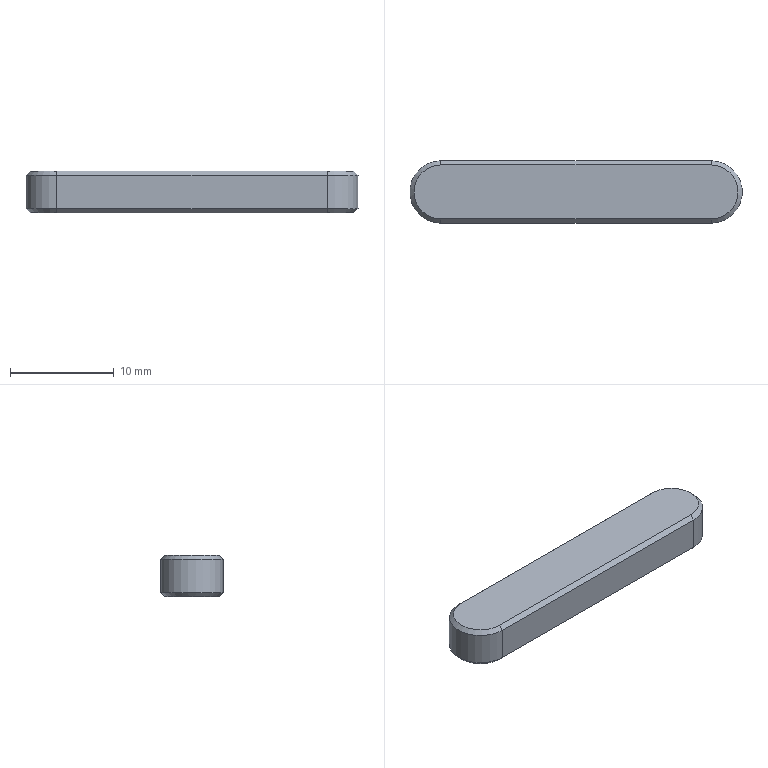Part | STEP file | ISO 2491 - A  6 x 4 x 32 | 1 solid | 14 faces | box 32 x 6 x 4 mm | volume 725.895 mm3 | plane 8 | cone 4 | cylinder 2 | commonest cylinder face diameters 6 x2
STEP:
#1=CARTESIAN_POINT('',(0.,0.,0.));
#2=DIRECTION('',(0.,0.,1.));
#3=DIRECTION('',(1.,0.,0.));
#4=AXIS2_PLACEMENT_3D('',#1,#2,#3);
#5=CARTESIAN_POINT('',(29.,-2.6,-2.5));
#6=VERTEX_POINT('',#5);
#7=CARTESIAN_POINT('',(29.,-3.,-2.1));
#8=VERTEX_POINT('',#7);
#9=CARTESIAN_POINT('',(29.,-2.6,-2.5));
#10=DIRECTION('',(0.,-0.7071,0.7071));
#11=VECTOR('',#10,1.);
#12=LINE('',#9,#11);
#13=CARTESIAN_POINT('',(9.5,-2.8,-2.3));
#14=DIRECTION('',(0.,-0.7071,-0.7071));
#15=DIRECTION('',(-1.,0.,0.));
#16=AXIS2_PLACEMENT_3D('',#13,#14,#15);
#17=PLANE('',#16);
#18=CARTESIAN_POINT('',(-19.5,0.2828));
#19=DIRECTION('',(0.,-1.));
#20=VECTOR('',#19,1.);
#21=LINE('',#18,#20);
#22=(GEOMETRIC_REPRESENTATION_CONTEXT(2)PARAMETRIC_REPRESENTATION_CONTEXT()REPRESENTATION_CONTEXT('',''));
#23=DEFINITIONAL_REPRESENTATION('',(#21),#22);
#24=PCURVE('',#17,#23);
#25=CARTESIAN_POINT('',(29.,0.,-2.3));
#26=DIRECTION('',(0.,0.,1.));
#27=DIRECTION('',(0.,1.,0.));
#28=AXIS2_PLACEMENT_3D('',#25,#26,#27);
#29=CONICAL_SURFACE('',#28,2.8,0.7854);
#30=CARTESIAN_POINT('',(3.142,-0.2));
#31=DIRECTION('',(0.,1.));
#32=VECTOR('',#31,1.);
#33=LINE('',#30,#32);
#34=(GEOMETRIC_REPRESENTATION_CONTEXT(2)PARAMETRIC_REPRESENTATION_CONTEXT()REPRESENTATION_CONTEXT('',''));
#35=DEFINITIONAL_REPRESENTATION('',(#33),#34);
#36=PCURVE('',#29,#35);
#37=SURFACE_CURVE('',#12,(#24,#36),.PCURVE_S1.);
#38=EDGE_CURVE('',#6,#8,#37,.T.);
#39=ORIENTED_EDGE('',*,*,#38,.T.);
#40=CARTESIAN_POINT('',(3.,-3.,-2.1));
#41=VERTEX_POINT('',#40);
#42=CARTESIAN_POINT('',(9.5,-3.,-2.1));
#43=DIRECTION('',(-1.,0.,0.));
#44=VECTOR('',#43,1.);
#45=LINE('',#42,#44);
#46=CARTESIAN_POINT('',(0.,-0.2828));
#47=DIRECTION('',(1.,0.));
#48=VECTOR('',#47,1.);
#49=LINE('',#46,#48);
#50=(GEOMETRIC_REPRESENTATION_CONTEXT(2)PARAMETRIC_REPRESENTATION_CONTEXT()REPRESENTATION_CONTEXT('',''));
#51=DEFINITIONAL_REPRESENTATION('',(#49),#50);
#52=PCURVE('',#17,#51);
#53=CARTESIAN_POINT('',(3.,-3.,0.));
#54=DIRECTION('',(0.,-1.,0.));
#55=DIRECTION('',(0.,0.,-1.));
#56=AXIS2_PLACEMENT_3D('',#53,#54,#55);
#57=PLANE('',#56);
#58=CARTESIAN_POINT('',(2.1,6.5));
#59=DIRECTION('',(0.,-1.));
#60=VECTOR('',#59,1.);
#61=LINE('',#58,#60);
#62=(GEOMETRIC_REPRESENTATION_CONTEXT(2)PARAMETRIC_REPRESENTATION_CONTEXT()REPRESENTATION_CONTEXT('',''));
#63=DEFINITIONAL_REPRESENTATION('',(#61),#62);
#64=PCURVE('',#57,#63);
#65=SURFACE_CURVE('',#45,(#52,#64),.PCURVE_S1.);
#66=EDGE_CURVE('',#8,#41,#65,.T.);
#67=ORIENTED_EDGE('',*,*,#66,.T.);
#68=CARTESIAN_POINT('',(3.,-2.6,-2.5));
#69=VERTEX_POINT('',#68);
#70=CARTESIAN_POINT('',(3.,-3.,-2.1));
#71=DIRECTION('',(0.,0.7071,-0.7071));
#72=VECTOR('',#71,1.);
#73=LINE('',#70,#72);
#74=CARTESIAN_POINT('',(6.5,-0.2828));
#75=DIRECTION('',(0.,1.));
#76=VECTOR('',#75,1.);
#77=LINE('',#74,#76);
#78=(GEOMETRIC_REPRESENTATION_CONTEXT(2)PARAMETRIC_REPRESENTATION_CONTEXT()REPRESENTATION_CONTEXT('',''));
#79=DEFINITIONAL_REPRESENTATION('',(#77),#78);
#80=PCURVE('',#17,#79);
#81=CARTESIAN_POINT('',(3.,0.,-2.3));
#82=DIRECTION('',(0.,0.,1.));
#83=DIRECTION('',(0.,-1.,0.));
#84=AXIS2_PLACEMENT_3D('',#81,#82,#83);
#85=CONICAL_SURFACE('',#84,2.8,0.7854);
#86=CARTESIAN_POINT('',(6.283,0.2));
#87=DIRECTION('',(0.,-1.));
#88=VECTOR('',#87,1.);
#89=LINE('',#86,#88);
#90=(GEOMETRIC_REPRESENTATION_CONTEXT(2)PARAMETRIC_REPRESENTATION_CONTEXT()REPRESENTATION_CONTEXT('',''));
#91=DEFINITIONAL_REPRESENTATION('',(#89),#90);
#92=PCURVE('',#85,#91);
#93=SURFACE_CURVE('',#73,(#80,#92),.PCURVE_S1.);
#94=EDGE_CURVE('',#41,#69,#93,.T.);
#95=ORIENTED_EDGE('',*,*,#94,.T.);
#96=CARTESIAN_POINT('',(9.5,-2.6,-2.5));
#97=DIRECTION('',(1.,0.,0.));
#98=VECTOR('',#97,1.);
#99=LINE('',#96,#98);
#100=CARTESIAN_POINT('',(0.,0.2828));
#101=DIRECTION('',(-1.,0.));
#102=VECTOR('',#101,1.);
#103=LINE('',#100,#102);
#104=(GEOMETRIC_REPRESENTATION_CONTEXT(2)PARAMETRIC_REPRESENTATION_CONTEXT()REPRESENTATION_CONTEXT('',''));
#105=DEFINITIONAL_REPRESENTATION('',(#103),#104);
#106=PCURVE('',#17,#105);
#107=CARTESIAN_POINT('',(16.,0.,-2.5));
#108=DIRECTION('',(0.,0.,1.));
#109=DIRECTION('',(1.,0.,0.));
#110=AXIS2_PLACEMENT_3D('',#107,#108,#109);
#111=PLANE('',#110);
#112=CARTESIAN_POINT('',(-6.5,-2.6));
#113=DIRECTION('',(1.,0.));
#114=VECTOR('',#113,1.);
#115=LINE('',#112,#114);
#116=(GEOMETRIC_REPRESENTATION_CONTEXT(2)PARAMETRIC_REPRESENTATION_CONTEXT()REPRESENTATION_CONTEXT('',''));
#117=DEFINITIONAL_REPRESENTATION('',(#115),#116);
#118=PCURVE('',#111,#117);
#119=SURFACE_CURVE('',#99,(#106,#118),.PCURVE_S1.);
#120=EDGE_CURVE('',#69,#6,#119,.T.);
#121=ORIENTED_EDGE('',*,*,#120,.T.);
#122=EDGE_LOOP('',(#39,#67,#95,#121));
#123=FACE_BOUND('',#122,.T.);
#124=ADVANCED_FACE('',(#123),#17,.T.);
#125=CARTESIAN_POINT('',(29.,2.6,-2.5));
#126=VERTEX_POINT('',#125);
#127=CARTESIAN_POINT('',(29.,3.,-2.1));
#128=VERTEX_POINT('',#127);
#129=CARTESIAN_POINT('',(29.,2.6,-2.5));
#130=DIRECTION('',(0.,0.7071,0.7071));
#131=VECTOR('',#130,1.);
#132=LINE('',#129,#131);
#133=CARTESIAN_POINT('',(6.283,-0.2));
#134=DIRECTION('',(0.,1.));
#135=VECTOR('',#134,1.);
#136=LINE('',#133,#135);
#137=(GEOMETRIC_REPRESENTATION_CONTEXT(2)PARAMETRIC_REPRESENTATION_CONTEXT()REPRESENTATION_CONTEXT('',''));
#138=DEFINITIONAL_REPRESENTATION('',(#136),#137);
#139=PCURVE('',#29,#138);
#140=CARTESIAN_POINT('',(22.5,2.8,-2.3));
#141=DIRECTION('',(0.,0.7071,-0.7071));
#142=DIRECTION('',(-1.,0.,0.));
#143=AXIS2_PLACEMENT_3D('',#140,#141,#142);
#144=PLANE('',#143);
#145=CARTESIAN_POINT('',(-6.5,-0.2828));
#146=DIRECTION('',(0.,1.));
#147=VECTOR('',#146,1.);
#148=LINE('',#145,#147);
#149=(GEOMETRIC_REPRESENTATION_CONTEXT(2)PARAMETRIC_REPRESENTATION_CONTEXT()REPRESENTATION_CONTEXT('',''));
#150=DEFINITIONAL_REPRESENTATION('',(#148),#149);
#151=PCURVE('',#144,#150);
#152=SURFACE_CURVE('',#132,(#139,#151),.PCURVE_S1.);
#153=EDGE_CURVE('',#126,#128,#152,.T.);
#154=ORIENTED_EDGE('',*,*,#153,.T.);
#155=CARTESIAN_POINT('',(29.,0.,-2.1));
#156=DIRECTION('',(0.,0.,-1.));
#157=DIRECTION('',(0.,1.,0.));
#158=AXIS2_PLACEMENT_3D('',#155,#156,#157);
#159=CIRCLE('',#158,3.);
#160=CARTESIAN_POINT('',(6.283,0.2));
#161=DIRECTION('',(-1.,0.));
#162=VECTOR('',#161,1.);
#163=LINE('',#160,#162);
#164=(GEOMETRIC_REPRESENTATION_CONTEXT(2)PARAMETRIC_REPRESENTATION_CONTEXT()REPRESENTATION_CONTEXT('',''));
#165=DEFINITIONAL_REPRESENTATION('',(#163),#164);
#166=PCURVE('',#29,#165);
#167=CARTESIAN_POINT('',(29.,0.,0.));
#168=DIRECTION('',(0.,0.,-1.));
#169=DIRECTION('',(0.,1.,0.));
#170=AXIS2_PLACEMENT_3D('',#167,#168,#169);
#171=CYLINDRICAL_SURFACE('',#170,3.);
#172=CARTESIAN_POINT('',(0.,2.1));
#173=DIRECTION('',(1.,0.));
#174=VECTOR('',#173,1.);
#175=LINE('',#172,#174);
#176=(GEOMETRIC_REPRESENTATION_CONTEXT(2)PARAMETRIC_REPRESENTATION_CONTEXT()REPRESENTATION_CONTEXT('',''));
#177=DEFINITIONAL_REPRESENTATION('',(#175),#176);
#178=PCURVE('',#171,#177);
#179=SURFACE_CURVE('',#159,(#166,#178),.PCURVE_S1.);
#180=EDGE_CURVE('',#128,#8,#179,.T.);
#181=ORIENTED_EDGE('',*,*,#180,.T.);
#182=ORIENTED_EDGE('',*,*,#38,.F.);
#183=CARTESIAN_POINT('',(29.,0.,-2.5));
#184=DIRECTION('',(0.,0.,1.));
#185=DIRECTION('',(0.,1.,0.));
#186=AXIS2_PLACEMENT_3D('',#183,#184,#185);
#187=CIRCLE('',#186,2.6);
#188=CARTESIAN_POINT('',(0.,-0.2));
#189=DIRECTION('',(1.,0.));
#190=VECTOR('',#189,1.);
#191=LINE('',#188,#190);
#192=(GEOMETRIC_REPRESENTATION_CONTEXT(2)PARAMETRIC_REPRESENTATION_CONTEXT()REPRESENTATION_CONTEXT('',''));
#193=DEFINITIONAL_REPRESENTATION('',(#191),#192);
#194=PCURVE('',#29,#193);
#195=CARTESIAN_POINT('',(13.,0.));
#196=DIRECTION('',(0.,1.));
#197=AXIS2_PLACEMENT_2D('',#195,#196);
#198=CIRCLE('',#197,2.6);
#199=(GEOMETRIC_REPRESENTATION_CONTEXT(2)PARAMETRIC_REPRESENTATION_CONTEXT()REPRESENTATION_CONTEXT('',''));
#200=DEFINITIONAL_REPRESENTATION('',(#198),#199);
#201=PCURVE('',#111,#200);
#202=SURFACE_CURVE('',#187,(#194,#201),.PCURVE_S1.);
#203=EDGE_CURVE('',#6,#126,#202,.T.);
#204=ORIENTED_EDGE('',*,*,#203,.T.);
#205=EDGE_LOOP('',(#154,#181,#182,#204));
#206=FACE_BOUND('',#205,.T.);
#207=ADVANCED_FACE('',(#206),#29,.T.);
#208=CARTESIAN_POINT('',(3.,3.,-2.1));
#209=VERTEX_POINT('',#208);
#210=CARTESIAN_POINT('',(3.,2.6,-2.5));
#211=VERTEX_POINT('',#210);
#212=CARTESIAN_POINT('',(3.,3.,-2.1));
#213=DIRECTION('',(0.,-0.7071,-0.7071));
#214=VECTOR('',#213,1.);
#215=LINE('',#212,#214);
#216=CARTESIAN_POINT('',(3.142,0.2));
#217=DIRECTION('',(0.,-1.));
#218=VECTOR('',#217,1.);
#219=LINE('',#216,#218);
#220=(GEOMETRIC_REPRESENTATION_CONTEXT(2)PARAMETRIC_REPRESENTATION_CONTEXT()REPRESENTATION_CONTEXT('',''));
#221=DEFINITIONAL_REPRESENTATION('',(#219),#220);
#222=PCURVE('',#85,#221);
#223=CARTESIAN_POINT('',(19.5,0.2828));
#224=DIRECTION('',(0.,-1.));
#225=VECTOR('',#224,1.);
#226=LINE('',#223,#225);
#227=(GEOMETRIC_REPRESENTATION_CONTEXT(2)PARAMETRIC_REPRESENTATION_CONTEXT()REPRESENTATION_CONTEXT('',''));
#228=DEFINITIONAL_REPRESENTATION('',(#226),#227);
#229=PCURVE('',#144,#228);
#230=SURFACE_CURVE('',#215,(#222,#229),.PCURVE_S1.);
#231=EDGE_CURVE('',#209,#211,#230,.T.);
#232=ORIENTED_EDGE('',*,*,#231,.T.);
#233=CARTESIAN_POINT('',(3.,0.,-2.5));
#234=DIRECTION('',(0.,0.,1.));
#235=DIRECTION('',(0.,-1.,0.));
#236=AXIS2_PLACEMENT_3D('',#233,#234,#235);
#237=CIRCLE('',#236,2.6);
#238=CARTESIAN_POINT('',(0.,-0.2));
#239=DIRECTION('',(1.,0.));
#240=VECTOR('',#239,1.);
#241=LINE('',#238,#240);
#242=(GEOMETRIC_REPRESENTATION_CONTEXT(2)PARAMETRIC_REPRESENTATION_CONTEXT()REPRESENTATION_CONTEXT('',''));
#243=DEFINITIONAL_REPRESENTATION('',(#241),#242);
#244=PCURVE('',#85,#243);
#245=CARTESIAN_POINT('',(-13.,0.));
#246=DIRECTION('',(0.,-1.));
#247=AXIS2_PLACEMENT_2D('',#245,#246);
#248=CIRCLE('',#247,2.6);
#249=(GEOMETRIC_REPRESENTATION_CONTEXT(2)PARAMETRIC_REPRESENTATION_CONTEXT()REPRESENTATION_CONTEXT('',''));
#250=DEFINITIONAL_REPRESENTATION('',(#248),#249);
#251=PCURVE('',#111,#250);
#252=SURFACE_CURVE('',#237,(#244,#251),.PCURVE_S1.);
#253=EDGE_CURVE('',#211,#69,#252,.T.);
#254=ORIENTED_EDGE('',*,*,#253,.T.);
#255=ORIENTED_EDGE('',*,*,#94,.F.);
#256=CARTESIAN_POINT('',(3.,0.,-2.1));
#257=DIRECTION('',(0.,0.,-1.));
#258=DIRECTION('',(0.,-1.,0.));
#259=AXIS2_PLACEMENT_3D('',#256,#257,#258);
#260=CIRCLE('',#259,3.);
#261=CARTESIAN_POINT('',(6.283,0.2));
#262=DIRECTION('',(-1.,0.));
#263=VECTOR('',#262,1.);
#264=LINE('',#261,#263);
#265=(GEOMETRIC_REPRESENTATION_CONTEXT(2)PARAMETRIC_REPRESENTATION_CONTEXT()REPRESENTATION_CONTEXT('',''));
#266=DEFINITIONAL_REPRESENTATION('',(#264),#265);
#267=PCURVE('',#85,#266);
#268=CARTESIAN_POINT('',(3.,0.,0.));
#269=DIRECTION('',(0.,0.,-1.));
#270=DIRECTION('',(0.,-1.,0.));
#271=AXIS2_PLACEMENT_3D('',#268,#269,#270);
#272=CYLINDRICAL_SURFACE('',#271,3.);
#273=CARTESIAN_POINT('',(0.,2.1));
#274=DIRECTION('',(1.,0.));
#275=VECTOR('',#274,1.);
#276=LINE('',#273,#275);
#277=(GEOMETRIC_REPRESENTATION_CONTEXT(2)PARAMETRIC_REPRESENTATION_CONTEXT()REPRESENTATION_CONTEXT('',''));
#278=DEFINITIONAL_REPRESENTATION('',(#276),#277);
#279=PCURVE('',#272,#278);
#280=SURFACE_CURVE('',#260,(#267,#279),.PCURVE_S1.);
#281=EDGE_CURVE('',#41,#209,#280,.T.);
#282=ORIENTED_EDGE('',*,*,#281,.T.);
#283=EDGE_LOOP('',(#232,#254,#255,#282));
#284=FACE_BOUND('',#283,.T.);
#285=ADVANCED_FACE('',(#284),#85,.T.);
#286=ORIENTED_EDGE('',*,*,#153,.F.);
#287=CARTESIAN_POINT('',(22.5,2.6,-2.5));
#288=DIRECTION('',(-1.,0.,0.));
#289=VECTOR('',#288,1.);
#290=LINE('',#287,#289);
#291=CARTESIAN_POINT('',(0.,-0.2828));
#292=DIRECTION('',(1.,0.));
#293=VECTOR('',#292,1.);
#294=LINE('',#291,#293);
#295=(GEOMETRIC_REPRESENTATION_CONTEXT(2)PARAMETRIC_REPRESENTATION_CONTEXT()REPRESENTATION_CONTEXT('',''));
#296=DEFINITIONAL_REPRESENTATION('',(#294),#295);
#297=PCURVE('',#144,#296);
#298=CARTESIAN_POINT('',(6.5,2.6));
#299=DIRECTION('',(-1.,0.));
#300=VECTOR('',#299,1.);
#301=LINE('',#298,#300);
#302=(GEOMETRIC_REPRESENTATION_CONTEXT(2)PARAMETRIC_REPRESENTATION_CONTEXT()REPRESENTATION_CONTEXT('',''));
#303=DEFINITIONAL_REPRESENTATION('',(#301),#302);
#304=PCURVE('',#111,#303);
#305=SURFACE_CURVE('',#290,(#297,#304),.PCURVE_S1.);
#306=EDGE_CURVE('',#126,#211,#305,.T.);
#307=ORIENTED_EDGE('',*,*,#306,.T.);
#308=ORIENTED_EDGE('',*,*,#231,.F.);
#309=CARTESIAN_POINT('',(22.5,3.,-2.1));
#310=DIRECTION('',(1.,0.,0.));
#311=VECTOR('',#310,1.);
#312=LINE('',#309,#311);
#313=CARTESIAN_POINT('',(0.,0.2828));
#314=DIRECTION('',(-1.,0.));
#315=VECTOR('',#314,1.);
#316=LINE('',#313,#315);
#317=(GEOMETRIC_REPRESENTATION_CONTEXT(2)PARAMETRIC_REPRESENTATION_CONTEXT()REPRESENTATION_CONTEXT('',''));
#318=DEFINITIONAL_REPRESENTATION('',(#316),#317);
#319=PCURVE('',#144,#318);
#320=CARTESIAN_POINT('',(29.,3.,0.));
#321=DIRECTION('',(0.,1.,0.));
#322=DIRECTION('',(0.,0.,1.));
#323=AXIS2_PLACEMENT_3D('',#320,#321,#322);
#324=PLANE('',#323);
#325=CARTESIAN_POINT('',(-2.1,-6.5));
#326=DIRECTION('',(0.,1.));
#327=VECTOR('',#326,1.);
#328=LINE('',#325,#327);
#329=(GEOMETRIC_REPRESENTATION_CONTEXT(2)PARAMETRIC_REPRESENTATION_CONTEXT()REPRESENTATION_CONTEXT('',''));
#330=DEFINITIONAL_REPRESENTATION('',(#328),#329);
#331=PCURVE('',#324,#330);
#332=SURFACE_CURVE('',#312,(#319,#331),.PCURVE_S1.);
#333=EDGE_CURVE('',#209,#128,#332,.T.);
#334=ORIENTED_EDGE('',*,*,#333,.T.);
#335=EDGE_LOOP('',(#286,#307,#308,#334));
#336=FACE_BOUND('',#335,.T.);
#337=ADVANCED_FACE('',(#336),#144,.T.);
#338=ORIENTED_EDGE('',*,*,#281,.F.);
#339=CARTESIAN_POINT('',(3.,-3.,1.1));
#340=VERTEX_POINT('',#339);
#341=CARTESIAN_POINT('',(3.,-3.,0.));
#342=DIRECTION('',(0.,0.,-1.));
#343=VECTOR('',#342,1.);
#344=LINE('',#341,#343);
#345=CARTESIAN_POINT('',(0.,0.));
#346=DIRECTION('',(0.,1.));
#347=VECTOR('',#346,1.);
#348=LINE('',#345,#347);
#349=(GEOMETRIC_REPRESENTATION_CONTEXT(2)PARAMETRIC_REPRESENTATION_CONTEXT()REPRESENTATION_CONTEXT('',''));
#350=DEFINITIONAL_REPRESENTATION('',(#348),#349);
#351=PCURVE('',#272,#350);
#352=CARTESIAN_POINT('',(0.,0.));
#353=DIRECTION('',(1.,0.));
#354=VECTOR('',#353,1.);
#355=LINE('',#352,#354);
#356=(GEOMETRIC_REPRESENTATION_CONTEXT(2)PARAMETRIC_REPRESENTATION_CONTEXT()REPRESENTATION_CONTEXT('',''));
#357=DEFINITIONAL_REPRESENTATION('',(#355),#356);
#358=PCURVE('',#57,#357);
#359=SURFACE_CURVE('',#344,(#351,#358),.PCURVE_S1.);
#360=EDGE_CURVE('',#340,#41,#359,.T.);
#361=ORIENTED_EDGE('',*,*,#360,.F.);
#362=CARTESIAN_POINT('',(3.,3.,1.1));
#363=VERTEX_POINT('',#362);
#364=CARTESIAN_POINT('',(3.,0.,1.1));
#365=DIRECTION('',(0.,0.,1.));
#366=DIRECTION('',(0.,-1.,0.));
#367=AXIS2_PLACEMENT_3D('',#364,#365,#366);
#368=CIRCLE('',#367,3.);
#369=CARTESIAN_POINT('',(6.283,-1.1));
#370=DIRECTION('',(-1.,0.));
#371=VECTOR('',#370,1.);
#372=LINE('',#369,#371);
#373=(GEOMETRIC_REPRESENTATION_CONTEXT(2)PARAMETRIC_REPRESENTATION_CONTEXT()REPRESENTATION_CONTEXT('',''));
#374=DEFINITIONAL_REPRESENTATION('',(#372),#373);
#375=PCURVE('',#272,#374);
#376=CARTESIAN_POINT('',(3.,0.,1.3));
#377=DIRECTION('',(0.,0.,-1.));
#378=DIRECTION('',(0.,-1.,0.));
#379=AXIS2_PLACEMENT_3D('',#376,#377,#378);
#380=CONICAL_SURFACE('',#379,2.8,0.7854);
#381=CARTESIAN_POINT('',(6.283,0.2));
#382=DIRECTION('',(-1.,0.));
#383=VECTOR('',#382,1.);
#384=LINE('',#381,#383);
#385=(GEOMETRIC_REPRESENTATION_CONTEXT(2)PARAMETRIC_REPRESENTATION_CONTEXT()REPRESENTATION_CONTEXT('',''));
#386=DEFINITIONAL_REPRESENTATION('',(#384),#385);
#387=PCURVE('',#380,#386);
#388=SURFACE_CURVE('',#368,(#375,#387),.PCURVE_S1.);
#389=EDGE_CURVE('',#363,#340,#388,.T.);
#390=ORIENTED_EDGE('',*,*,#389,.F.);
#391=CARTESIAN_POINT('',(3.,3.,0.));
#392=DIRECTION('',(0.,0.,1.));
#393=VECTOR('',#392,1.);
#394=LINE('',#391,#393);
#395=CARTESIAN_POINT('',(3.142,0.));
#396=DIRECTION('',(0.,-1.));
#397=VECTOR('',#396,1.);
#398=LINE('',#395,#397);
#399=(GEOMETRIC_REPRESENTATION_CONTEXT(2)PARAMETRIC_REPRESENTATION_CONTEXT()REPRESENTATION_CONTEXT('',''));
#400=DEFINITIONAL_REPRESENTATION('',(#398),#399);
#401=PCURVE('',#272,#400);
#402=CARTESIAN_POINT('',(0.,-26.));
#403=DIRECTION('',(1.,0.));
#404=VECTOR('',#403,1.);
#405=LINE('',#402,#404);
#406=(GEOMETRIC_REPRESENTATION_CONTEXT(2)PARAMETRIC_REPRESENTATION_CONTEXT()REPRESENTATION_CONTEXT('',''));
#407=DEFINITIONAL_REPRESENTATION('',(#405),#406);
#408=PCURVE('',#324,#407);
#409=SURFACE_CURVE('',#394,(#401,#408),.PCURVE_S1.);
#410=EDGE_CURVE('',#209,#363,#409,.T.);
#411=ORIENTED_EDGE('',*,*,#410,.F.);
#412=EDGE_LOOP('',(#338,#361,#390,#411));
#413=FACE_BOUND('',#412,.T.);
#414=ADVANCED_FACE('',(#413),#272,.T.);
#415=ORIENTED_EDGE('',*,*,#66,.F.);
#416=CARTESIAN_POINT('',(29.,-3.,1.1));
#417=VERTEX_POINT('',#416);
#418=CARTESIAN_POINT('',(29.,-3.,0.));
#419=DIRECTION('',(0.,0.,-1.));
#420=VECTOR('',#419,1.);
#421=LINE('',#418,#420);
#422=CARTESIAN_POINT('',(0.,26.));
#423=DIRECTION('',(1.,0.));
#424=VECTOR('',#423,1.);
#425=LINE('',#422,#424);
#426=(GEOMETRIC_REPRESENTATION_CONTEXT(2)PARAMETRIC_REPRESENTATION_CONTEXT()REPRESENTATION_CONTEXT('',''));
#427=DEFINITIONAL_REPRESENTATION('',(#425),#426);
#428=PCURVE('',#57,#427);
#429=CARTESIAN_POINT('',(3.142,0.));
#430=DIRECTION('',(0.,1.));
#431=VECTOR('',#430,1.);
#432=LINE('',#429,#431);
#433=(GEOMETRIC_REPRESENTATION_CONTEXT(2)PARAMETRIC_REPRESENTATION_CONTEXT()REPRESENTATION_CONTEXT('',''));
#434=DEFINITIONAL_REPRESENTATION('',(#432),#433);
#435=PCURVE('',#171,#434);
#436=SURFACE_CURVE('',#421,(#428,#435),.PCURVE_S1.);
#437=EDGE_CURVE('',#417,#8,#436,.T.);
#438=ORIENTED_EDGE('',*,*,#437,.F.);
#439=CARTESIAN_POINT('',(9.5,-3.,1.1));
#440=DIRECTION('',(1.,0.,0.));
#441=VECTOR('',#440,1.);
#442=LINE('',#439,#441);
#443=CARTESIAN_POINT('',(-1.1,6.5));
#444=DIRECTION('',(0.,1.));
#445=VECTOR('',#444,1.);
#446=LINE('',#443,#445);
#447=(GEOMETRIC_REPRESENTATION_CONTEXT(2)PARAMETRIC_REPRESENTATION_CONTEXT()REPRESENTATION_CONTEXT('',''));
#448=DEFINITIONAL_REPRESENTATION('',(#446),#447);
#449=PCURVE('',#57,#448);
#450=CARTESIAN_POINT('',(9.5,-2.8,1.3));
#451=DIRECTION('',(0.,-0.7071,0.7071));
#452=DIRECTION('',(1.,0.,0.));
#453=AXIS2_PLACEMENT_3D('',#450,#451,#452);
#454=PLANE('',#453);
#455=CARTESIAN_POINT('',(0.,-0.2828));
#456=DIRECTION('',(1.,0.));
#457=VECTOR('',#456,1.);
#458=LINE('',#455,#457);
#459=(GEOMETRIC_REPRESENTATION_CONTEXT(2)PARAMETRIC_REPRESENTATION_CONTEXT()REPRESENTATION_CONTEXT('',''));
#460=DEFINITIONAL_REPRESENTATION('',(#458),#459);
#461=PCURVE('',#454,#460);
#462=SURFACE_CURVE('',#442,(#449,#461),.PCURVE_S1.);
#463=EDGE_CURVE('',#340,#417,#462,.T.);
#464=ORIENTED_EDGE('',*,*,#463,.F.);
#465=ORIENTED_EDGE('',*,*,#360,.T.);
#466=EDGE_LOOP('',(#415,#438,#464,#465));
#467=FACE_BOUND('',#466,.T.);
#468=ADVANCED_FACE('',(#467),#57,.T.);
#469=ORIENTED_EDGE('',*,*,#120,.F.);
#470=ORIENTED_EDGE('',*,*,#253,.F.);
#471=ORIENTED_EDGE('',*,*,#306,.F.);
#472=ORIENTED_EDGE('',*,*,#203,.F.);
#473=EDGE_LOOP('',(#469,#470,#471,#472));
#474=FACE_BOUND('',#473,.T.);
#475=ADVANCED_FACE('',(#474),#111,.F.);
#476=CARTESIAN_POINT('',(3.,-2.6,1.5));
#477=VERTEX_POINT('',#476);
#478=CARTESIAN_POINT('',(3.,-3.,1.1));
#479=DIRECTION('',(0.,0.7071,0.7071));
#480=VECTOR('',#479,1.);
#481=LINE('',#478,#480);
#482=CARTESIAN_POINT('',(0.,0.2));
#483=DIRECTION('',(0.,-1.));
#484=VECTOR('',#483,1.);
#485=LINE('',#482,#484);
#486=(GEOMETRIC_REPRESENTATION_CONTEXT(2)PARAMETRIC_REPRESENTATION_CONTEXT()REPRESENTATION_CONTEXT('',''));
#487=DEFINITIONAL_REPRESENTATION('',(#485),#486);
#488=PCURVE('',#380,#487);
#489=CARTESIAN_POINT('',(-6.5,-0.2828));
#490=DIRECTION('',(0.,1.));
#491=VECTOR('',#490,1.);
#492=LINE('',#489,#491);
#493=(GEOMETRIC_REPRESENTATION_CONTEXT(2)PARAMETRIC_REPRESENTATION_CONTEXT()REPRESENTATION_CONTEXT('',''));
#494=DEFINITIONAL_REPRESENTATION('',(#492),#493);
#495=PCURVE('',#454,#494);
#496=SURFACE_CURVE('',#481,(#488,#495),.PCURVE_S1.);
#497=EDGE_CURVE('',#340,#477,#496,.T.);
#498=ORIENTED_EDGE('',*,*,#497,.T.);
#499=CARTESIAN_POINT('',(3.,2.6,1.5));
#500=VERTEX_POINT('',#499);
#501=CARTESIAN_POINT('',(3.,0.,1.5));
#502=DIRECTION('',(0.,0.,-1.));
#503=DIRECTION('',(0.,-1.,0.));
#504=AXIS2_PLACEMENT_3D('',#501,#502,#503);
#505=CIRCLE('',#504,2.6);
#506=CARTESIAN_POINT('',(0.,-0.2));
#507=DIRECTION('',(1.,0.));
#508=VECTOR('',#507,1.);
#509=LINE('',#506,#508);
#510=(GEOMETRIC_REPRESENTATION_CONTEXT(2)PARAMETRIC_REPRESENTATION_CONTEXT()REPRESENTATION_CONTEXT('',''));
#511=DEFINITIONAL_REPRESENTATION('',(#509),#510);
#512=PCURVE('',#380,#511);
#513=CARTESIAN_POINT('',(16.,0.,1.5));
#514=DIRECTION('',(0.,0.,1.));
#515=DIRECTION('',(1.,0.,0.));
#516=AXIS2_PLACEMENT_3D('',#513,#514,#515);
#517=PLANE('',#516);
#518=CARTESIAN_POINT('',(-13.,-2.6));
#519=CARTESIAN_POINT('',(-17.503,-2.6));
#520=CARTESIAN_POINT('',(-15.252,1.3));
#521=CARTESIAN_POINT('',(-13.,5.2));
#522=CARTESIAN_POINT('',(-10.748,1.3));
#523=CARTESIAN_POINT('',(-8.497,-2.6));
#524=CARTESIAN_POINT('',(-13.,-2.6));
#525=(BOUNDED_CURVE()B_SPLINE_CURVE(2,(#518,#519,#520,#521,#522,#523,#524),.UNSPECIFIED.,.T.,.F.)B_SPLINE_CURVE_WITH_KNOTS((1,2,2,2,2,1),(-2.094,0.,2.094,4.189,6.283,8.378),.UNSPECIFIED.)CURVE()GEOMETRIC_REPRESENTATION_ITEM()RATIONAL_B_SPLINE_CURVE((1.,0.5,1.,0.5,1.,0.5,1.))REPRESENTATION_ITEM(''));
#526=(GEOMETRIC_REPRESENTATION_CONTEXT(2)PARAMETRIC_REPRESENTATION_CONTEXT()REPRESENTATION_CONTEXT('',''));
#527=DEFINITIONAL_REPRESENTATION('',(#525),#526);
#528=PCURVE('',#517,#527);
#529=SURFACE_CURVE('',#505,(#512,#528),.PCURVE_S1.);
#530=EDGE_CURVE('',#477,#500,#529,.T.);
#531=ORIENTED_EDGE('',*,*,#530,.T.);
#532=CARTESIAN_POINT('',(3.,2.6,1.5));
#533=DIRECTION('',(0.,0.7071,-0.7071));
#534=VECTOR('',#533,1.);
#535=LINE('',#532,#534);
#536=CARTESIAN_POINT('',(3.142,-0.2));
#537=DIRECTION('',(0.,1.));
#538=VECTOR('',#537,1.);
#539=LINE('',#536,#538);
#540=(GEOMETRIC_REPRESENTATION_CONTEXT(2)PARAMETRIC_REPRESENTATION_CONTEXT()REPRESENTATION_CONTEXT('',''));
#541=DEFINITIONAL_REPRESENTATION('',(#539),#540);
#542=PCURVE('',#380,#541);
#543=CARTESIAN_POINT('',(22.5,2.8,1.3));
#544=DIRECTION('',(0.,0.7071,0.7071));
#545=DIRECTION('',(1.,0.,0.));
#546=AXIS2_PLACEMENT_3D('',#543,#544,#545);
#547=PLANE('',#546);
#548=CARTESIAN_POINT('',(-19.5,-0.2828));
#549=DIRECTION('',(0.,1.));
#550=VECTOR('',#549,1.);
#551=LINE('',#548,#550);
#552=(GEOMETRIC_REPRESENTATION_CONTEXT(2)PARAMETRIC_REPRESENTATION_CONTEXT()REPRESENTATION_CONTEXT('',''));
#553=DEFINITIONAL_REPRESENTATION('',(#551),#552);
#554=PCURVE('',#547,#553);
#555=SURFACE_CURVE('',#535,(#542,#554),.PCURVE_S1.);
#556=EDGE_CURVE('',#500,#363,#555,.T.);
#557=ORIENTED_EDGE('',*,*,#556,.T.);
#558=ORIENTED_EDGE('',*,*,#389,.T.);
#559=EDGE_LOOP('',(#498,#531,#557,#558));
#560=FACE_BOUND('',#559,.T.);
#561=ADVANCED_FACE('',(#560),#380,.T.);
#562=CARTESIAN_POINT('',(29.,-2.6,1.5));
#563=VERTEX_POINT('',#562);
#564=CARTESIAN_POINT('',(29.,-3.,1.1));
#565=DIRECTION('',(0.,0.7071,0.7071));
#566=VECTOR('',#565,1.);
#567=LINE('',#564,#566);
#568=CARTESIAN_POINT('',(19.5,-0.2828));
#569=DIRECTION('',(0.,1.));
#570=VECTOR('',#569,1.);
#571=LINE('',#568,#570);
#572=(GEOMETRIC_REPRESENTATION_CONTEXT(2)PARAMETRIC_REPRESENTATION_CONTEXT()REPRESENTATION_CONTEXT('',''));
#573=DEFINITIONAL_REPRESENTATION('',(#571),#572);
#574=PCURVE('',#454,#573);
#575=CARTESIAN_POINT('',(29.,0.,1.3));
#576=DIRECTION('',(0.,0.,-1.));
#577=DIRECTION('',(0.,1.,0.));
#578=AXIS2_PLACEMENT_3D('',#575,#576,#577);
#579=CONICAL_SURFACE('',#578,2.8,0.7854);
#580=CARTESIAN_POINT('',(3.142,0.2));
#581=DIRECTION('',(0.,-1.));
#582=VECTOR('',#581,1.);
#583=LINE('',#580,#582);
#584=(GEOMETRIC_REPRESENTATION_CONTEXT(2)PARAMETRIC_REPRESENTATION_CONTEXT()REPRESENTATION_CONTEXT('',''));
#585=DEFINITIONAL_REPRESENTATION('',(#583),#584);
#586=PCURVE('',#579,#585);
#587=SURFACE_CURVE('',#567,(#574,#586),.PCURVE_S1.);
#588=EDGE_CURVE('',#417,#563,#587,.T.);
#589=ORIENTED_EDGE('',*,*,#588,.T.);
#590=CARTESIAN_POINT('',(9.5,-2.6,1.5));
#591=DIRECTION('',(-1.,0.,0.));
#592=VECTOR('',#591,1.);
#593=LINE('',#590,#592);
#594=CARTESIAN_POINT('',(0.,0.2828));
#595=DIRECTION('',(-1.,0.));
#596=VECTOR('',#595,1.);
#597=LINE('',#594,#596);
#598=(GEOMETRIC_REPRESENTATION_CONTEXT(2)PARAMETRIC_REPRESENTATION_CONTEXT()REPRESENTATION_CONTEXT('',''));
#599=DEFINITIONAL_REPRESENTATION('',(#597),#598);
#600=PCURVE('',#454,#599);
#601=CARTESIAN_POINT('',(-6.5,-2.6));
#602=DIRECTION('',(-1.,0.));
#603=VECTOR('',#602,1.);
#604=LINE('',#601,#603);
#605=(GEOMETRIC_REPRESENTATION_CONTEXT(2)PARAMETRIC_REPRESENTATION_CONTEXT()REPRESENTATION_CONTEXT('',''));
#606=DEFINITIONAL_REPRESENTATION('',(#604),#605);
#607=PCURVE('',#517,#606);
#608=SURFACE_CURVE('',#593,(#600,#607),.PCURVE_S1.);
#609=EDGE_CURVE('',#563,#477,#608,.T.);
#610=ORIENTED_EDGE('',*,*,#609,.T.);
#611=ORIENTED_EDGE('',*,*,#497,.F.);
#612=ORIENTED_EDGE('',*,*,#463,.T.);
#613=EDGE_LOOP('',(#589,#610,#611,#612));
#614=FACE_BOUND('',#613,.T.);
#615=ADVANCED_FACE('',(#614),#454,.T.);
#616=CARTESIAN_POINT('',(29.,2.6,1.5));
#617=VERTEX_POINT('',#616);
#618=CARTESIAN_POINT('',(29.,3.,1.1));
#619=VERTEX_POINT('',#618);
#620=CARTESIAN_POINT('',(29.,2.6,1.5));
#621=DIRECTION('',(0.,0.7071,-0.7071));
#622=VECTOR('',#621,1.);
#623=LINE('',#620,#622);
#624=CARTESIAN_POINT('',(6.5,-0.2828));
#625=DIRECTION('',(0.,1.));
#626=VECTOR('',#625,1.);
#627=LINE('',#624,#626);
#628=(GEOMETRIC_REPRESENTATION_CONTEXT(2)PARAMETRIC_REPRESENTATION_CONTEXT()REPRESENTATION_CONTEXT('',''));
#629=DEFINITIONAL_REPRESENTATION('',(#627),#628);
#630=PCURVE('',#547,#629);
#631=CARTESIAN_POINT('',(0.,-0.2));
#632=DIRECTION('',(0.,1.));
#633=VECTOR('',#632,1.);
#634=LINE('',#631,#633);
#635=(GEOMETRIC_REPRESENTATION_CONTEXT(2)PARAMETRIC_REPRESENTATION_CONTEXT()REPRESENTATION_CONTEXT('',''));
#636=DEFINITIONAL_REPRESENTATION('',(#634),#635);
#637=PCURVE('',#579,#636);
#638=SURFACE_CURVE('',#623,(#630,#637),.PCURVE_S1.);
#639=EDGE_CURVE('',#617,#619,#638,.T.);
#640=ORIENTED_EDGE('',*,*,#639,.T.);
#641=CARTESIAN_POINT('',(22.5,3.,1.1));
#642=DIRECTION('',(-1.,0.,0.));
#643=VECTOR('',#642,1.);
#644=LINE('',#641,#643);
#645=CARTESIAN_POINT('',(0.,0.2828));
#646=DIRECTION('',(-1.,0.));
#647=VECTOR('',#646,1.);
#648=LINE('',#645,#647);
#649=(GEOMETRIC_REPRESENTATION_CONTEXT(2)PARAMETRIC_REPRESENTATION_CONTEXT()REPRESENTATION_CONTEXT('',''));
#650=DEFINITIONAL_REPRESENTATION('',(#648),#649);
#651=PCURVE('',#547,#650);
#652=CARTESIAN_POINT('',(1.1,-6.5));
#653=DIRECTION('',(0.,-1.));
#654=VECTOR('',#653,1.);
#655=LINE('',#652,#654);
#656=(GEOMETRIC_REPRESENTATION_CONTEXT(2)PARAMETRIC_REPRESENTATION_CONTEXT()REPRESENTATION_CONTEXT('',''));
#657=DEFINITIONAL_REPRESENTATION('',(#655),#656);
#658=PCURVE('',#324,#657);
#659=SURFACE_CURVE('',#644,(#651,#658),.PCURVE_S1.);
#660=EDGE_CURVE('',#619,#363,#659,.T.);
#661=ORIENTED_EDGE('',*,*,#660,.T.);
#662=ORIENTED_EDGE('',*,*,#556,.F.);
#663=CARTESIAN_POINT('',(22.5,2.6,1.5));
#664=DIRECTION('',(1.,0.,0.));
#665=VECTOR('',#664,1.);
#666=LINE('',#663,#665);
#667=CARTESIAN_POINT('',(0.,-0.2828));
#668=DIRECTION('',(1.,0.));
#669=VECTOR('',#668,1.);
#670=LINE('',#667,#669);
#671=(GEOMETRIC_REPRESENTATION_CONTEXT(2)PARAMETRIC_REPRESENTATION_CONTEXT()REPRESENTATION_CONTEXT('',''));
#672=DEFINITIONAL_REPRESENTATION('',(#670),#671);
#673=PCURVE('',#547,#672);
#674=CARTESIAN_POINT('',(6.5,2.6));
#675=DIRECTION('',(1.,0.));
#676=VECTOR('',#675,1.);
#677=LINE('',#674,#676);
#678=(GEOMETRIC_REPRESENTATION_CONTEXT(2)PARAMETRIC_REPRESENTATION_CONTEXT()REPRESENTATION_CONTEXT('',''));
#679=DEFINITIONAL_REPRESENTATION('',(#677),#678);
#680=PCURVE('',#517,#679);
#681=SURFACE_CURVE('',#666,(#673,#680),.PCURVE_S1.);
#682=EDGE_CURVE('',#500,#617,#681,.T.);
#683=ORIENTED_EDGE('',*,*,#682,.T.);
#684=EDGE_LOOP('',(#640,#661,#662,#683));
#685=FACE_BOUND('',#684,.T.);
#686=ADVANCED_FACE('',(#685),#547,.T.);
#687=ORIENTED_EDGE('',*,*,#588,.F.);
#688=CARTESIAN_POINT('',(29.,0.,1.1));
#689=DIRECTION('',(0.,0.,1.));
#690=DIRECTION('',(0.,1.,0.));
#691=AXIS2_PLACEMENT_3D('',#688,#689,#690);
#692=CIRCLE('',#691,3.);
#693=CARTESIAN_POINT('',(6.283,0.2));
#694=DIRECTION('',(-1.,0.));
#695=VECTOR('',#694,1.);
#696=LINE('',#693,#695);
#697=(GEOMETRIC_REPRESENTATION_CONTEXT(2)PARAMETRIC_REPRESENTATION_CONTEXT()REPRESENTATION_CONTEXT('',''));
#698=DEFINITIONAL_REPRESENTATION('',(#696),#697);
#699=PCURVE('',#579,#698);
#700=CARTESIAN_POINT('',(6.283,-1.1));
#701=DIRECTION('',(-1.,0.));
#702=VECTOR('',#701,1.);
#703=LINE('',#700,#702);
#704=(GEOMETRIC_REPRESENTATION_CONTEXT(2)PARAMETRIC_REPRESENTATION_CONTEXT()REPRESENTATION_CONTEXT('',''));
#705=DEFINITIONAL_REPRESENTATION('',(#703),#704);
#706=PCURVE('',#171,#705);
#707=SURFACE_CURVE('',#692,(#699,#706),.PCURVE_S1.);
#708=EDGE_CURVE('',#417,#619,#707,.T.);
#709=ORIENTED_EDGE('',*,*,#708,.T.);
#710=ORIENTED_EDGE('',*,*,#639,.F.);
#711=CARTESIAN_POINT('',(29.,0.,1.5));
#712=DIRECTION('',(0.,0.,-1.));
#713=DIRECTION('',(0.,1.,0.));
#714=AXIS2_PLACEMENT_3D('',#711,#712,#713);
#715=CIRCLE('',#714,2.6);
#716=CARTESIAN_POINT('',(0.,-0.2));
#717=DIRECTION('',(1.,0.));
#718=VECTOR('',#717,1.);
#719=LINE('',#716,#718);
#720=(GEOMETRIC_REPRESENTATION_CONTEXT(2)PARAMETRIC_REPRESENTATION_CONTEXT()REPRESENTATION_CONTEXT('',''));
#721=DEFINITIONAL_REPRESENTATION('',(#719),#720);
#722=PCURVE('',#579,#721);
#723=CARTESIAN_POINT('',(13.,2.6));
#724=CARTESIAN_POINT('',(17.503,2.6));
#725=CARTESIAN_POINT('',(15.252,-1.3));
#726=CARTESIAN_POINT('',(13.,-5.2));
#727=CARTESIAN_POINT('',(10.748,-1.3));
#728=CARTESIAN_POINT('',(8.497,2.6));
#729=CARTESIAN_POINT('',(13.,2.6));
#730=(BOUNDED_CURVE()B_SPLINE_CURVE(2,(#723,#724,#725,#726,#727,#728,#729),.UNSPECIFIED.,.T.,.F.)B_SPLINE_CURVE_WITH_KNOTS((1,2,2,2,2,1),(-2.094,0.,2.094,4.189,6.283,8.378),.UNSPECIFIED.)CURVE()GEOMETRIC_REPRESENTATION_ITEM()RATIONAL_B_SPLINE_CURVE((1.,0.5,1.,0.5,1.,0.5,1.))REPRESENTATION_ITEM(''));
#731=(GEOMETRIC_REPRESENTATION_CONTEXT(2)PARAMETRIC_REPRESENTATION_CONTEXT()REPRESENTATION_CONTEXT('',''));
#732=DEFINITIONAL_REPRESENTATION('',(#730),#731);
#733=PCURVE('',#517,#732);
#734=SURFACE_CURVE('',#715,(#722,#733),.PCURVE_S1.);
#735=EDGE_CURVE('',#617,#563,#734,.T.);
#736=ORIENTED_EDGE('',*,*,#735,.T.);
#737=EDGE_LOOP('',(#687,#709,#710,#736));
#738=FACE_BOUND('',#737,.T.);
#739=ADVANCED_FACE('',(#738),#579,.T.);
#740=ORIENTED_EDGE('',*,*,#530,.F.);
#741=ORIENTED_EDGE('',*,*,#609,.F.);
#742=ORIENTED_EDGE('',*,*,#735,.F.);
#743=ORIENTED_EDGE('',*,*,#682,.F.);
#744=EDGE_LOOP('',(#740,#741,#742,#743));
#745=FACE_BOUND('',#744,.T.);
#746=ADVANCED_FACE('',(#745),#517,.T.);
#747=ORIENTED_EDGE('',*,*,#333,.F.);
#748=ORIENTED_EDGE('',*,*,#410,.T.);
#749=ORIENTED_EDGE('',*,*,#660,.F.);
#750=CARTESIAN_POINT('',(29.,3.,0.));
#751=DIRECTION('',(0.,0.,-1.));
#752=VECTOR('',#751,1.);
#753=LINE('',#750,#752);
#754=CARTESIAN_POINT('',(0.,0.));
#755=DIRECTION('',(-1.,0.));
#756=VECTOR('',#755,1.);
#757=LINE('',#754,#756);
#758=(GEOMETRIC_REPRESENTATION_CONTEXT(2)PARAMETRIC_REPRESENTATION_CONTEXT()REPRESENTATION_CONTEXT('',''));
#759=DEFINITIONAL_REPRESENTATION('',(#757),#758);
#760=PCURVE('',#324,#759);
#761=CARTESIAN_POINT('',(0.,0.));
#762=DIRECTION('',(0.,1.));
#763=VECTOR('',#762,1.);
#764=LINE('',#761,#763);
#765=(GEOMETRIC_REPRESENTATION_CONTEXT(2)PARAMETRIC_REPRESENTATION_CONTEXT()REPRESENTATION_CONTEXT('',''));
#766=DEFINITIONAL_REPRESENTATION('',(#764),#765);
#767=PCURVE('',#171,#766);
#768=SURFACE_CURVE('',#753,(#760,#767),.PCURVE_S1.);
#769=EDGE_CURVE('',#619,#128,#768,.T.);
#770=ORIENTED_EDGE('',*,*,#769,.T.);
#771=EDGE_LOOP('',(#747,#748,#749,#770));
#772=FACE_BOUND('',#771,.T.);
#773=ADVANCED_FACE('',(#772),#324,.T.);
#774=ORIENTED_EDGE('',*,*,#180,.F.);
#775=ORIENTED_EDGE('',*,*,#769,.F.);
#776=ORIENTED_EDGE('',*,*,#708,.F.);
#777=ORIENTED_EDGE('',*,*,#437,.T.);
#778=EDGE_LOOP('',(#774,#775,#776,#777));
#779=FACE_BOUND('',#778,.T.);
#780=ADVANCED_FACE('',(#779),#171,.T.);
#781=CLOSED_SHELL('',(#124,#207,#285,#337,#414,#468,#475,#561,#615,#686,#739,#746,#773,#780));
#782=MANIFOLD_SOLID_BREP('',#781);
#783=(LENGTH_UNIT()NAMED_UNIT(*)SI_UNIT(.MILLI.,.METRE.));
#784=UNCERTAINTY_MEASURE_WITH_UNIT(LENGTH_MEASURE(0.0000001),#783,'','');
#785=(NAMED_UNIT(*)PLANE_ANGLE_UNIT()SI_UNIT($,.RADIAN.));
#786=(NAMED_UNIT(*)SI_UNIT($,.STERADIAN.)SOLID_ANGLE_UNIT());
#787=(GEOMETRIC_REPRESENTATION_CONTEXT(3)GLOBAL_UNCERTAINTY_ASSIGNED_CONTEXT((#784))GLOBAL_UNIT_ASSIGNED_CONTEXT((#783,#785,#786))REPRESENTATION_CONTEXT('',''));
#788=ADVANCED_BREP_SHAPE_REPRESENTATION('',(#4,#782),#787);